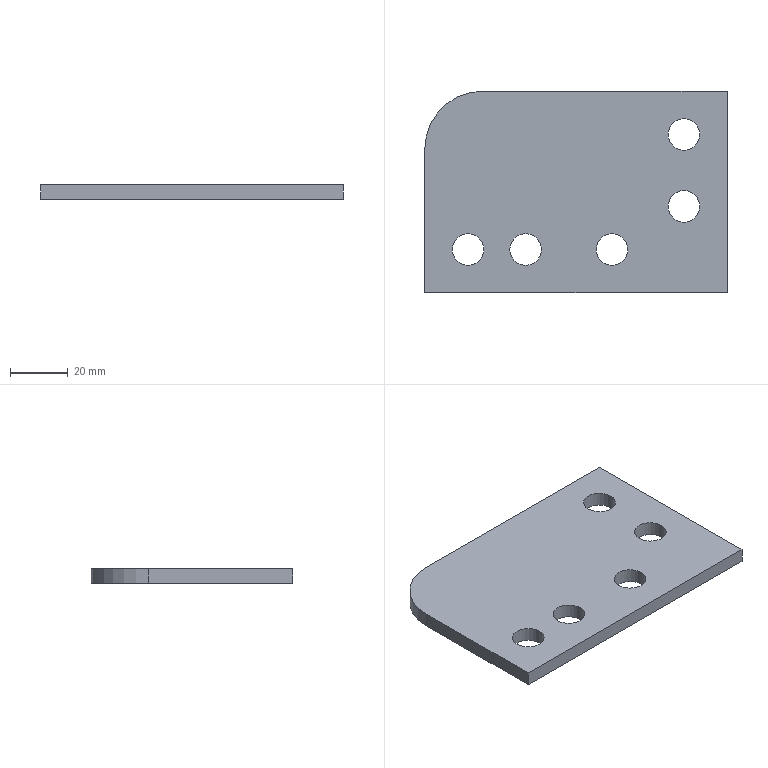Part | NX | features solid 2 | 1 solid | 12 faces | box 105 x 70 x 5 mm | volume 33945 mm3 | plane 6 | cylinder 6 | commonest cylinder face diameters 11 x5 40 x1
STEP:
#1=CARTESIAN_POINT('',(-310.,200.,114.));
#2=VERTEX_POINT('',#1);
#3=CARTESIAN_POINT('',(-310.,250.,114.));
#4=VERTEX_POINT('',#3);
#5=CARTESIAN_POINT('',(-310.,200.,114.));
#6=DIRECTION('',(0.,1.,0.));
#7=VECTOR('',#6,1000.);
#8=LINE('',#5,#7);
#9=EDGE_CURVE('',#2,#4,#8,.T.);
#10=ORIENTED_EDGE('',*,*,#9,.T.);
#11=CARTESIAN_POINT('',(-310.,250.,109.));
#12=VERTEX_POINT('',#11);
#13=CARTESIAN_POINT('',(-310.,250.,114.));
#14=DIRECTION('',(0.,0.,-1.));
#15=VECTOR('',#14,1000.);
#16=LINE('',#13,#15);
#17=EDGE_CURVE('',#4,#12,#16,.T.);
#18=ORIENTED_EDGE('',*,*,#17,.T.);
#19=CARTESIAN_POINT('',(-310.,200.,109.));
#20=VERTEX_POINT('',#19);
#21=CARTESIAN_POINT('',(-310.,200.,109.));
#22=DIRECTION('',(0.,1.,0.));
#23=VECTOR('',#22,1000.);
#24=LINE('',#21,#23);
#25=EDGE_CURVE('',#20,#12,#24,.T.);
#26=ORIENTED_EDGE('',*,*,#25,.F.);
#27=CARTESIAN_POINT('',(-310.,200.,114.));
#28=DIRECTION('',(0.,0.,-1.));
#29=VECTOR('',#28,1000.);
#30=LINE('',#27,#29);
#31=EDGE_CURVE('',#2,#20,#30,.T.);
#32=ORIENTED_EDGE('',*,*,#31,.F.);
#33=EDGE_LOOP('',(#10,#18,#26,#32));
#34=FACE_BOUND('',#33,.T.);
#35=CARTESIAN_POINT('',(-310.,200.,114.));
#36=DIRECTION('',(-1.,0.,0.));
#37=DIRECTION('',(0.,0.,1.));
#38=AXIS2_PLACEMENT_3D('',#35,#36,#37);
#39=PLANE('',#38);
#40=ADVANCED_FACE('',(#34),#39,.T.);
#41=CARTESIAN_POINT('',(-290.,270.,109.));
#42=VERTEX_POINT('',#41);
#43=CARTESIAN_POINT('',(-205.,270.,109.));
#44=VERTEX_POINT('',#43);
#45=CARTESIAN_POINT('',(-310.,270.,109.));
#46=DIRECTION('',(1.,0.,0.));
#47=VECTOR('',#46,1000.);
#48=LINE('',#45,#47);
#49=EDGE_CURVE('',#42,#44,#48,.T.);
#50=ORIENTED_EDGE('',*,*,#49,.F.);
#51=CARTESIAN_POINT('',(-290.,270.,114.));
#52=VERTEX_POINT('',#51);
#53=CARTESIAN_POINT('',(-290.,270.,114.));
#54=DIRECTION('',(0.,0.,-1.));
#55=VECTOR('',#54,1000.);
#56=LINE('',#53,#55);
#57=EDGE_CURVE('',#42,#52,#56,.F.);
#58=ORIENTED_EDGE('',*,*,#57,.T.);
#59=CARTESIAN_POINT('',(-205.,270.,114.));
#60=VERTEX_POINT('',#59);
#61=CARTESIAN_POINT('',(-310.,270.,114.));
#62=DIRECTION('',(1.,0.,0.));
#63=VECTOR('',#62,1000.);
#64=LINE('',#61,#63);
#65=EDGE_CURVE('',#52,#60,#64,.T.);
#66=ORIENTED_EDGE('',*,*,#65,.T.);
#67=CARTESIAN_POINT('',(-205.,270.,114.));
#68=DIRECTION('',(0.,0.,-1.));
#69=VECTOR('',#68,1000.);
#70=LINE('',#67,#69);
#71=EDGE_CURVE('',#60,#44,#70,.T.);
#72=ORIENTED_EDGE('',*,*,#71,.T.);
#73=EDGE_LOOP('',(#50,#58,#66,#72));
#74=FACE_BOUND('',#73,.T.);
#75=CARTESIAN_POINT('',(-310.,270.,114.));
#76=DIRECTION('',(0.,1.,0.));
#77=DIRECTION('',(0.,0.,1.));
#78=AXIS2_PLACEMENT_3D('',#75,#76,#77);
#79=PLANE('',#78);
#80=ADVANCED_FACE('',(#74),#79,.T.);
#81=CARTESIAN_POINT('',(-205.,200.,109.));
#82=VERTEX_POINT('',#81);
#83=CARTESIAN_POINT('',(-205.,265.,109.));
#84=DIRECTION('',(0.,1.,0.));
#85=VECTOR('',#84,1000.);
#86=LINE('',#83,#85);
#87=EDGE_CURVE('',#82,#44,#86,.T.);
#88=ORIENTED_EDGE('',*,*,#87,.T.);
#89=ORIENTED_EDGE('',*,*,#71,.F.);
#90=CARTESIAN_POINT('',(-205.,200.,114.));
#91=VERTEX_POINT('',#90);
#92=CARTESIAN_POINT('',(-205.,265.,114.));
#93=DIRECTION('',(0.,1.,0.));
#94=VECTOR('',#93,1000.);
#95=LINE('',#92,#94);
#96=EDGE_CURVE('',#91,#60,#95,.T.);
#97=ORIENTED_EDGE('',*,*,#96,.F.);
#98=CARTESIAN_POINT('',(-205.,200.,114.));
#99=DIRECTION('',(0.,0.,-1.));
#100=VECTOR('',#99,1000.);
#101=LINE('',#98,#100);
#102=EDGE_CURVE('',#91,#82,#101,.T.);
#103=ORIENTED_EDGE('',*,*,#102,.T.);
#104=EDGE_LOOP('',(#88,#89,#97,#103));
#105=FACE_BOUND('',#104,.T.);
#106=CARTESIAN_POINT('',(-205.,200.,114.));
#107=DIRECTION('',(-1.,0.,0.));
#108=DIRECTION('',(0.,0.,1.));
#109=AXIS2_PLACEMENT_3D('',#106,#107,#108);
#110=PLANE('',#109);
#111=ADVANCED_FACE('',(#105),#110,.F.);
#112=CARTESIAN_POINT('',(-310.,200.,109.));
#113=DIRECTION('',(1.,0.,0.));
#114=VECTOR('',#113,1000.);
#115=LINE('',#112,#114);
#116=EDGE_CURVE('',#20,#82,#115,.T.);
#117=ORIENTED_EDGE('',*,*,#116,.T.);
#118=ORIENTED_EDGE('',*,*,#102,.F.);
#119=CARTESIAN_POINT('',(-310.,200.,114.));
#120=DIRECTION('',(1.,0.,0.));
#121=VECTOR('',#120,1000.);
#122=LINE('',#119,#121);
#123=EDGE_CURVE('',#2,#91,#122,.T.);
#124=ORIENTED_EDGE('',*,*,#123,.F.);
#125=ORIENTED_EDGE('',*,*,#31,.T.);
#126=EDGE_LOOP('',(#117,#118,#124,#125));
#127=FACE_BOUND('',#126,.T.);
#128=CARTESIAN_POINT('',(-310.,200.,114.));
#129=DIRECTION('',(0.,1.,0.));
#130=DIRECTION('',(0.,0.,1.));
#131=AXIS2_PLACEMENT_3D('',#128,#129,#130);
#132=PLANE('',#131);
#133=ADVANCED_FACE('',(#127),#132,.F.);
#134=CARTESIAN_POINT('',(-225.5,230.,114.));
#135=VERTEX_POINT('',#134);
#136=CARTESIAN_POINT('',(-220.,230.,114.));
#137=DIRECTION('',(0.,0.,-1.));
#138=DIRECTION('',(-1.,0.,0.));
#139=AXIS2_PLACEMENT_3D('',#136,#137,#138);
#140=CIRCLE('',#139,5.5);
#141=EDGE_CURVE('',#135,#135,#140,.T.);
#142=ORIENTED_EDGE('',*,*,#141,.T.);
#143=EDGE_LOOP('',(#142));
#144=FACE_BOUND('',#143,.T.);
#145=CARTESIAN_POINT('',(-280.5,215.,114.));
#146=VERTEX_POINT('',#145);
#147=CARTESIAN_POINT('',(-275.,215.,114.));
#148=DIRECTION('',(0.,0.,-1.));
#149=DIRECTION('',(-1.,0.,0.));
#150=AXIS2_PLACEMENT_3D('',#147,#148,#149);
#151=CIRCLE('',#150,5.5);
#152=EDGE_CURVE('',#146,#146,#151,.T.);
#153=ORIENTED_EDGE('',*,*,#152,.T.);
#154=EDGE_LOOP('',(#153));
#155=FACE_BOUND('',#154,.T.);
#156=CARTESIAN_POINT('',(-300.5,215.,114.));
#157=VERTEX_POINT('',#156);
#158=CARTESIAN_POINT('',(-295.,215.,114.));
#159=DIRECTION('',(0.,0.,-1.));
#160=DIRECTION('',(-1.,0.,0.));
#161=AXIS2_PLACEMENT_3D('',#158,#159,#160);
#162=CIRCLE('',#161,5.5);
#163=EDGE_CURVE('',#157,#157,#162,.T.);
#164=ORIENTED_EDGE('',*,*,#163,.T.);
#165=EDGE_LOOP('',(#164));
#166=FACE_BOUND('',#165,.T.);
#167=CARTESIAN_POINT('',(-250.5,215.,114.));
#168=VERTEX_POINT('',#167);
#169=CARTESIAN_POINT('',(-245.,215.,114.));
#170=DIRECTION('',(0.,0.,-1.));
#171=DIRECTION('',(-1.,0.,0.));
#172=AXIS2_PLACEMENT_3D('',#169,#170,#171);
#173=CIRCLE('',#172,5.5);
#174=EDGE_CURVE('',#168,#168,#173,.T.);
#175=ORIENTED_EDGE('',*,*,#174,.T.);
#176=EDGE_LOOP('',(#175));
#177=FACE_BOUND('',#176,.T.);
#178=CARTESIAN_POINT('',(-225.5,255.,114.));
#179=VERTEX_POINT('',#178);
#180=CARTESIAN_POINT('',(-220.,255.,114.));
#181=DIRECTION('',(0.,0.,-1.));
#182=DIRECTION('',(-1.,0.,0.));
#183=AXIS2_PLACEMENT_3D('',#180,#181,#182);
#184=CIRCLE('',#183,5.5);
#185=EDGE_CURVE('',#179,#179,#184,.T.);
#186=ORIENTED_EDGE('',*,*,#185,.T.);
#187=EDGE_LOOP('',(#186));
#188=FACE_BOUND('',#187,.T.);
#189=ORIENTED_EDGE('',*,*,#65,.F.);
#190=CARTESIAN_POINT('',(-290.,250.,114.));
#191=DIRECTION('',(0.,0.,-1.));
#192=DIRECTION('',(-1.,0.,0.));
#193=AXIS2_PLACEMENT_3D('',#190,#191,#192);
#194=CIRCLE('',#193,20.);
#195=EDGE_CURVE('',#52,#4,#194,.F.);
#196=ORIENTED_EDGE('',*,*,#195,.T.);
#197=ORIENTED_EDGE('',*,*,#9,.F.);
#198=ORIENTED_EDGE('',*,*,#123,.T.);
#199=ORIENTED_EDGE('',*,*,#96,.T.);
#200=EDGE_LOOP('',(#189,#196,#197,#198,#199));
#201=FACE_BOUND('',#200,.T.);
#202=CARTESIAN_POINT('',(-310.,265.,114.));
#203=DIRECTION('',(0.,0.,-1.));
#204=DIRECTION('',(-1.,0.,0.));
#205=AXIS2_PLACEMENT_3D('',#202,#203,#204);
#206=PLANE('',#205);
#207=ADVANCED_FACE('',(#144,#155,#166,#177,#188,#201),#206,.F.);
#208=CARTESIAN_POINT('',(-225.5,230.,109.));
#209=VERTEX_POINT('',#208);
#210=CARTESIAN_POINT('',(-220.,230.,109.));
#211=DIRECTION('',(0.,0.,-1.));
#212=DIRECTION('',(-1.,0.,0.));
#213=AXIS2_PLACEMENT_3D('',#210,#211,#212);
#214=CIRCLE('',#213,5.5);
#215=EDGE_CURVE('',#209,#209,#214,.T.);
#216=ORIENTED_EDGE('',*,*,#215,.F.);
#217=EDGE_LOOP('',(#216));
#218=FACE_BOUND('',#217,.T.);
#219=CARTESIAN_POINT('',(-280.5,215.,109.));
#220=VERTEX_POINT('',#219);
#221=CARTESIAN_POINT('',(-275.,215.,109.));
#222=DIRECTION('',(0.,0.,-1.));
#223=DIRECTION('',(-1.,0.,0.));
#224=AXIS2_PLACEMENT_3D('',#221,#222,#223);
#225=CIRCLE('',#224,5.5);
#226=EDGE_CURVE('',#220,#220,#225,.T.);
#227=ORIENTED_EDGE('',*,*,#226,.F.);
#228=EDGE_LOOP('',(#227));
#229=FACE_BOUND('',#228,.T.);
#230=CARTESIAN_POINT('',(-300.5,215.,109.));
#231=VERTEX_POINT('',#230);
#232=CARTESIAN_POINT('',(-295.,215.,109.));
#233=DIRECTION('',(0.,0.,-1.));
#234=DIRECTION('',(-1.,0.,0.));
#235=AXIS2_PLACEMENT_3D('',#232,#233,#234);
#236=CIRCLE('',#235,5.5);
#237=EDGE_CURVE('',#231,#231,#236,.T.);
#238=ORIENTED_EDGE('',*,*,#237,.F.);
#239=EDGE_LOOP('',(#238));
#240=FACE_BOUND('',#239,.T.);
#241=CARTESIAN_POINT('',(-250.5,215.,109.));
#242=VERTEX_POINT('',#241);
#243=CARTESIAN_POINT('',(-245.,215.,109.));
#244=DIRECTION('',(0.,0.,-1.));
#245=DIRECTION('',(-1.,0.,0.));
#246=AXIS2_PLACEMENT_3D('',#243,#244,#245);
#247=CIRCLE('',#246,5.5);
#248=EDGE_CURVE('',#242,#242,#247,.T.);
#249=ORIENTED_EDGE('',*,*,#248,.F.);
#250=EDGE_LOOP('',(#249));
#251=FACE_BOUND('',#250,.T.);
#252=CARTESIAN_POINT('',(-225.5,255.,109.));
#253=VERTEX_POINT('',#252);
#254=CARTESIAN_POINT('',(-220.,255.,109.));
#255=DIRECTION('',(0.,0.,-1.));
#256=DIRECTION('',(-1.,0.,0.));
#257=AXIS2_PLACEMENT_3D('',#254,#255,#256);
#258=CIRCLE('',#257,5.5);
#259=EDGE_CURVE('',#253,#253,#258,.T.);
#260=ORIENTED_EDGE('',*,*,#259,.F.);
#261=EDGE_LOOP('',(#260));
#262=FACE_BOUND('',#261,.T.);
#263=ORIENTED_EDGE('',*,*,#25,.T.);
#264=CARTESIAN_POINT('',(-290.,250.,109.));
#265=DIRECTION('',(0.,0.,-1.));
#266=DIRECTION('',(-1.,0.,0.));
#267=AXIS2_PLACEMENT_3D('',#264,#265,#266);
#268=CIRCLE('',#267,20.);
#269=EDGE_CURVE('',#12,#42,#268,.T.);
#270=ORIENTED_EDGE('',*,*,#269,.T.);
#271=ORIENTED_EDGE('',*,*,#49,.T.);
#272=ORIENTED_EDGE('',*,*,#87,.F.);
#273=ORIENTED_EDGE('',*,*,#116,.F.);
#274=EDGE_LOOP('',(#263,#270,#271,#272,#273));
#275=FACE_BOUND('',#274,.T.);
#276=CARTESIAN_POINT('',(-310.,265.,109.));
#277=DIRECTION('',(0.,0.,-1.));
#278=DIRECTION('',(-1.,0.,0.));
#279=AXIS2_PLACEMENT_3D('',#276,#277,#278);
#280=PLANE('',#279);
#281=ADVANCED_FACE('',(#218,#229,#240,#251,#262,#275),#280,.T.);
#282=ORIENTED_EDGE('',*,*,#259,.T.);
#283=EDGE_LOOP('',(#282));
#284=FACE_BOUND('',#283,.T.);
#285=ORIENTED_EDGE('',*,*,#185,.F.);
#286=EDGE_LOOP('',(#285));
#287=FACE_BOUND('',#286,.T.);
#288=CARTESIAN_POINT('',(-220.,255.,-111.));
#289=DIRECTION('',(0.,0.,1.));
#290=DIRECTION('',(1.,0.,0.));
#291=AXIS2_PLACEMENT_3D('',#288,#289,#290);
#292=CYLINDRICAL_SURFACE('',#291,5.5);
#293=ADVANCED_FACE('',(#284,#287),#292,.F.);
#294=ORIENTED_EDGE('',*,*,#248,.T.);
#295=EDGE_LOOP('',(#294));
#296=FACE_BOUND('',#295,.T.);
#297=ORIENTED_EDGE('',*,*,#174,.F.);
#298=EDGE_LOOP('',(#297));
#299=FACE_BOUND('',#298,.T.);
#300=CARTESIAN_POINT('',(-245.,215.,-111.));
#301=DIRECTION('',(0.,0.,1.));
#302=DIRECTION('',(1.,0.,0.));
#303=AXIS2_PLACEMENT_3D('',#300,#301,#302);
#304=CYLINDRICAL_SURFACE('',#303,5.5);
#305=ADVANCED_FACE('',(#296,#299),#304,.F.);
#306=ORIENTED_EDGE('',*,*,#237,.T.);
#307=EDGE_LOOP('',(#306));
#308=FACE_BOUND('',#307,.T.);
#309=ORIENTED_EDGE('',*,*,#163,.F.);
#310=EDGE_LOOP('',(#309));
#311=FACE_BOUND('',#310,.T.);
#312=CARTESIAN_POINT('',(-295.,215.,-111.));
#313=DIRECTION('',(0.,0.,1.));
#314=DIRECTION('',(1.,0.,0.));
#315=AXIS2_PLACEMENT_3D('',#312,#313,#314);
#316=CYLINDRICAL_SURFACE('',#315,5.5);
#317=ADVANCED_FACE('',(#308,#311),#316,.F.);
#318=ORIENTED_EDGE('',*,*,#226,.T.);
#319=EDGE_LOOP('',(#318));
#320=FACE_BOUND('',#319,.T.);
#321=ORIENTED_EDGE('',*,*,#152,.F.);
#322=EDGE_LOOP('',(#321));
#323=FACE_BOUND('',#322,.T.);
#324=CARTESIAN_POINT('',(-275.,215.,-121.));
#325=DIRECTION('',(0.,0.,1.));
#326=DIRECTION('',(1.,0.,0.));
#327=AXIS2_PLACEMENT_3D('',#324,#325,#326);
#328=CYLINDRICAL_SURFACE('',#327,5.5);
#329=ADVANCED_FACE('',(#320,#323),#328,.F.);
#330=ORIENTED_EDGE('',*,*,#215,.T.);
#331=EDGE_LOOP('',(#330));
#332=FACE_BOUND('',#331,.T.);
#333=ORIENTED_EDGE('',*,*,#141,.F.);
#334=EDGE_LOOP('',(#333));
#335=FACE_BOUND('',#334,.T.);
#336=CARTESIAN_POINT('',(-220.,230.,-121.));
#337=DIRECTION('',(0.,0.,1.));
#338=DIRECTION('',(1.,0.,0.));
#339=AXIS2_PLACEMENT_3D('',#336,#337,#338);
#340=CYLINDRICAL_SURFACE('',#339,5.5);
#341=ADVANCED_FACE('',(#332,#335),#340,.F.);
#342=ORIENTED_EDGE('',*,*,#195,.F.);
#343=ORIENTED_EDGE('',*,*,#57,.F.);
#344=ORIENTED_EDGE('',*,*,#269,.F.);
#345=ORIENTED_EDGE('',*,*,#17,.F.);
#346=EDGE_LOOP('',(#342,#343,#344,#345));
#347=FACE_BOUND('',#346,.T.);
#348=CARTESIAN_POINT('',(-290.,250.,114.));
#349=DIRECTION('',(0.,0.,-1.));
#350=DIRECTION('',(-1.,0.,0.));
#351=AXIS2_PLACEMENT_3D('',#348,#349,#350);
#352=CYLINDRICAL_SURFACE('',#351,20.);
#353=ADVANCED_FACE('',(#347),#352,.T.);
#354=CLOSED_SHELL('',(#40,#80,#111,#133,#207,#281,#293,#305,#317,#329,#341,#353));
#355=MANIFOLD_SOLID_BREP('',#354);
#356=(LENGTH_UNIT()NAMED_UNIT(*)SI_UNIT(.MILLI.,.METRE.));
#357=UNCERTAINTY_MEASURE_WITH_UNIT(LENGTH_MEASURE(0.00001),#356,'','');
#358=(NAMED_UNIT(*)PLANE_ANGLE_UNIT()SI_UNIT($,.RADIAN.));
#359=(NAMED_UNIT(*)SI_UNIT($,.STERADIAN.)SOLID_ANGLE_UNIT());
#360=(GEOMETRIC_REPRESENTATION_CONTEXT(3)GLOBAL_UNCERTAINTY_ASSIGNED_CONTEXT((#357))GLOBAL_UNIT_ASSIGNED_CONTEXT((#356,#358,#359))REPRESENTATION_CONTEXT('',''));
#361=ADVANCED_BREP_SHAPE_REPRESENTATION('',(#355),#360);